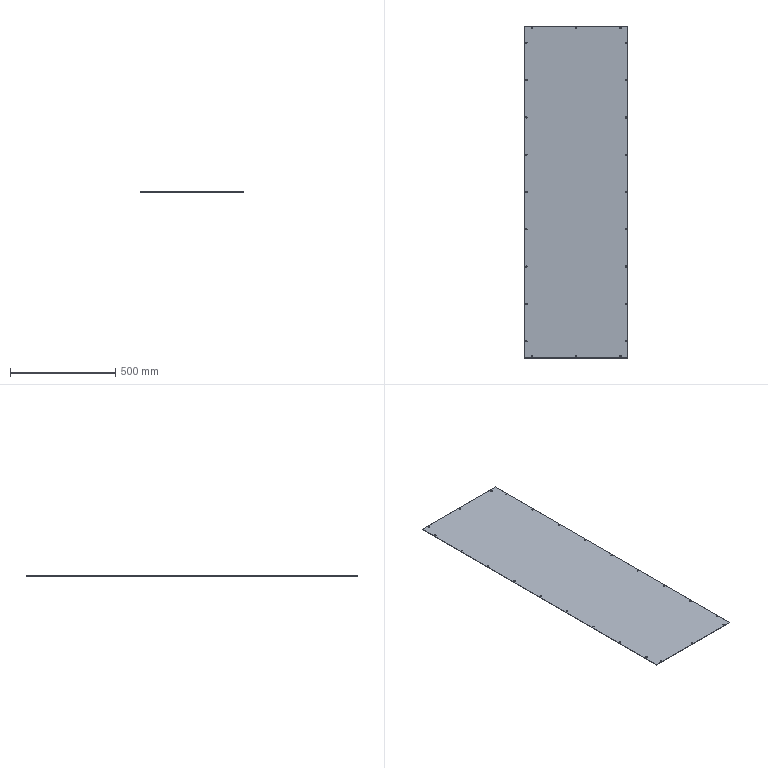Part | SolidWorks | 1 solid | 54 faces | box 492 x 1578 x 2 mm | volume 1551159 mm3 | cylinder 48 | plane 6 | commonest cylinder face diameters 6.5 x48